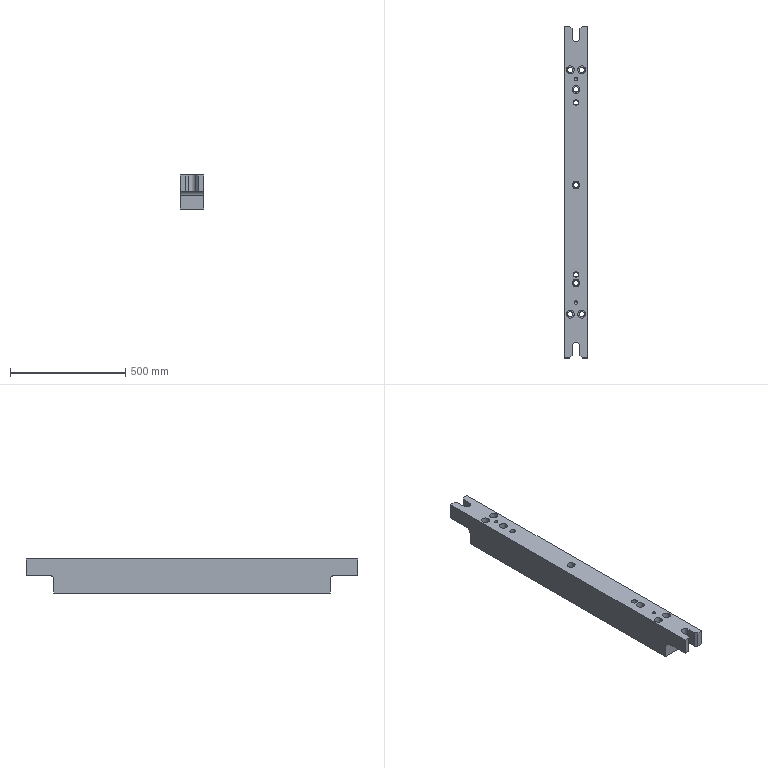Part | STEP file | lll_id2470_x_t | 1 solid | 55 faces | box 100 x 1440 x 147.5 mm | volume 18182535 mm3 | plane 29 | cylinder 24 | cone 2 | commonest cylinder face diameters 23.009 x7 34.008 x7 14.506 x2 20 x2 24 x2 34 x2
STEP:
#1=CARTESIAN_POINT('',(3774.688,-480.,370.));
#2=VERTEX_POINT('',#1);
#3=CARTESIAN_POINT('',(3767.435,-480.,370.));
#4=DIRECTION('',(0.,0.,-1.));
#5=DIRECTION('',(1.,0.,0.));
#6=AXIS2_PLACEMENT_3D('',#3,#4,#5);
#7=CIRCLE('',#6,7.253);
#8=EDGE_CURVE('',#2,#2,#7,.T.);
#9=ORIENTED_EDGE('',*,*,#8,.T.);
#10=EDGE_LOOP('',(#9));
#11=FACE_BOUND('',#10,.T.);
#12=CARTESIAN_POINT('',(3750.431,-395.,370.));
#13=VERTEX_POINT('',#12);
#14=CARTESIAN_POINT('',(3767.435,-395.,370.));
#15=DIRECTION('',(0.,0.,-1.));
#16=DIRECTION('',(-1.,0.,0.));
#17=AXIS2_PLACEMENT_3D('',#14,#15,#16);
#18=CIRCLE('',#17,17.004);
#19=EDGE_CURVE('',#13,#13,#18,.T.);
#20=ORIENTED_EDGE('',*,*,#19,.T.);
#21=EDGE_LOOP('',(#20));
#22=FACE_BOUND('',#21,.T.);
#23=CARTESIAN_POINT('',(3775.431,-530.,370.));
#24=VERTEX_POINT('',#23);
#25=CARTESIAN_POINT('',(3792.435,-530.,370.));
#26=DIRECTION('',(0.,0.,-1.));
#27=DIRECTION('',(-1.,0.,0.));
#28=AXIS2_PLACEMENT_3D('',#25,#26,#27);
#29=CIRCLE('',#28,17.004);
#30=EDGE_CURVE('',#24,#24,#29,.T.);
#31=ORIENTED_EDGE('',*,*,#30,.T.);
#32=EDGE_LOOP('',(#31));
#33=FACE_BOUND('',#32,.T.);
#34=CARTESIAN_POINT('',(3725.431,-530.,370.));
#35=VERTEX_POINT('',#34);
#36=CARTESIAN_POINT('',(3742.435,-530.,370.));
#37=DIRECTION('',(0.,0.,-1.));
#38=DIRECTION('',(-1.,0.,0.));
#39=AXIS2_PLACEMENT_3D('',#36,#37,#38);
#40=CIRCLE('',#39,17.004);
#41=EDGE_CURVE('',#35,#35,#40,.T.);
#42=ORIENTED_EDGE('',*,*,#41,.T.);
#43=EDGE_LOOP('',(#42));
#44=FACE_BOUND('',#43,.T.);
#45=CARTESIAN_POINT('',(3755.435,388.,370.));
#46=VERTEX_POINT('',#45);
#47=CARTESIAN_POINT('',(3767.435,388.,370.));
#48=DIRECTION('',(0.,0.,-1.));
#49=DIRECTION('',(-1.,0.,0.));
#50=AXIS2_PLACEMENT_3D('',#47,#48,#49);
#51=CIRCLE('',#50,12.);
#52=EDGE_CURVE('',#46,#46,#51,.T.);
#53=ORIENTED_EDGE('',*,*,#52,.T.);
#54=EDGE_LOOP('',(#53));
#55=FACE_BOUND('',#54,.T.);
#56=CARTESIAN_POINT('',(3784.439,30.,370.));
#57=VERTEX_POINT('',#56);
#58=CARTESIAN_POINT('',(3767.435,30.,370.));
#59=DIRECTION('',(0.,0.,-1.));
#60=DIRECTION('',(1.,0.,0.));
#61=AXIS2_PLACEMENT_3D('',#58,#59,#60);
#62=CIRCLE('',#61,17.004);
#63=EDGE_CURVE('',#57,#57,#62,.T.);
#64=ORIENTED_EDGE('',*,*,#63,.T.);
#65=EDGE_LOOP('',(#64));
#66=FACE_BOUND('',#65,.T.);
#67=CARTESIAN_POINT('',(3784.439,445.,370.));
#68=VERTEX_POINT('',#67);
#69=CARTESIAN_POINT('',(3767.435,445.,370.));
#70=DIRECTION('',(0.,0.,-1.));
#71=DIRECTION('',(1.,0.,0.));
#72=AXIS2_PLACEMENT_3D('',#69,#70,#71);
#73=CIRCLE('',#72,17.004);
#74=EDGE_CURVE('',#68,#68,#73,.T.);
#75=ORIENTED_EDGE('',*,*,#74,.T.);
#76=EDGE_LOOP('',(#75));
#77=FACE_BOUND('',#76,.T.);
#78=CARTESIAN_POINT('',(3740.435,-720.,370.));
#79=VERTEX_POINT('',#78);
#80=CARTESIAN_POINT('',(3717.435,-720.,370.));
#81=VERTEX_POINT('',#80);
#82=CARTESIAN_POINT('',(1551.12,-720.,370.));
#83=DIRECTION('',(-1.,0.,0.));
#84=VECTOR('',#83,1.);
#85=LINE('',#82,#84);
#86=EDGE_CURVE('',#79,#81,#85,.T.);
#87=ORIENTED_EDGE('',*,*,#86,.F.);
#88=CARTESIAN_POINT('',(3750.435,-710.,370.));
#89=VERTEX_POINT('',#88);
#90=CARTESIAN_POINT('',(3750.435,-710.,370.));
#91=DIRECTION('',(0.7071,0.7071,0.));
#92=VECTOR('',#91,1.);
#93=LINE('',#90,#92);
#94=EDGE_CURVE('',#79,#89,#93,.T.);
#95=ORIENTED_EDGE('',*,*,#94,.T.);
#96=CARTESIAN_POINT('',(3750.435,-670.,370.));
#97=VERTEX_POINT('',#96);
#98=CARTESIAN_POINT('',(3750.435,120.,370.));
#99=DIRECTION('',(0.,-1.,0.));
#100=VECTOR('',#99,1.);
#101=LINE('',#98,#100);
#102=EDGE_CURVE('',#97,#89,#101,.T.);
#103=ORIENTED_EDGE('',*,*,#102,.F.);
#104=CARTESIAN_POINT('',(3784.435,-670.,370.));
#105=VERTEX_POINT('',#104);
#106=CARTESIAN_POINT('',(3767.435,-670.,370.));
#107=DIRECTION('',(0.,0.,1.));
#108=DIRECTION('',(1.,0.,0.));
#109=AXIS2_PLACEMENT_3D('',#106,#107,#108);
#110=CIRCLE('',#109,17.);
#111=EDGE_CURVE('',#105,#97,#110,.T.);
#112=ORIENTED_EDGE('',*,*,#111,.F.);
#113=CARTESIAN_POINT('',(3784.435,-710.,370.));
#114=VERTEX_POINT('',#113);
#115=CARTESIAN_POINT('',(3784.435,120.,370.));
#116=DIRECTION('',(0.,1.,0.));
#117=VECTOR('',#116,1.);
#118=LINE('',#115,#117);
#119=EDGE_CURVE('',#114,#105,#118,.T.);
#120=ORIENTED_EDGE('',*,*,#119,.F.);
#121=CARTESIAN_POINT('',(3794.435,-720.,370.));
#122=VERTEX_POINT('',#121);
#123=CARTESIAN_POINT('',(3784.435,-710.,370.));
#124=DIRECTION('',(0.7071,-0.7071,0.));
#125=VECTOR('',#124,1.);
#126=LINE('',#123,#125);
#127=EDGE_CURVE('',#114,#122,#126,.T.);
#128=ORIENTED_EDGE('',*,*,#127,.T.);
#129=CARTESIAN_POINT('',(3817.435,-720.,370.));
#130=VERTEX_POINT('',#129);
#131=CARTESIAN_POINT('',(1551.12,-720.,370.));
#132=DIRECTION('',(-1.,0.,0.));
#133=VECTOR('',#132,1.);
#134=LINE('',#131,#133);
#135=EDGE_CURVE('',#130,#122,#134,.T.);
#136=ORIENTED_EDGE('',*,*,#135,.F.);
#137=CARTESIAN_POINT('',(3817.435,720.,370.));
#138=VERTEX_POINT('',#137);
#139=CARTESIAN_POINT('',(3817.435,0.,370.));
#140=DIRECTION('',(0.,-1.,0.));
#141=VECTOR('',#140,1.);
#142=LINE('',#139,#141);
#143=EDGE_CURVE('',#138,#130,#142,.T.);
#144=ORIENTED_EDGE('',*,*,#143,.F.);
#145=CARTESIAN_POINT('',(3794.435,720.,370.));
#146=VERTEX_POINT('',#145);
#147=CARTESIAN_POINT('',(1551.12,720.,370.));
#148=DIRECTION('',(1.,0.,0.));
#149=VECTOR('',#148,1.);
#150=LINE('',#147,#149);
#151=EDGE_CURVE('',#146,#138,#150,.T.);
#152=ORIENTED_EDGE('',*,*,#151,.F.);
#153=CARTESIAN_POINT('',(3784.435,710.,370.));
#154=VERTEX_POINT('',#153);
#155=CARTESIAN_POINT('',(3750.935,676.5,370.));
#156=DIRECTION('',(0.7071,0.7071,0.));
#157=VECTOR('',#156,1.);
#158=LINE('',#155,#157);
#159=EDGE_CURVE('',#154,#146,#158,.T.);
#160=ORIENTED_EDGE('',*,*,#159,.F.);
#161=CARTESIAN_POINT('',(3784.435,670.,370.));
#162=VERTEX_POINT('',#161);
#163=CARTESIAN_POINT('',(3784.435,-120.,370.));
#164=DIRECTION('',(0.,-1.,0.));
#165=VECTOR('',#164,1.);
#166=LINE('',#163,#165);
#167=EDGE_CURVE('',#154,#162,#166,.T.);
#168=ORIENTED_EDGE('',*,*,#167,.T.);
#169=CARTESIAN_POINT('',(3750.435,670.,370.));
#170=VERTEX_POINT('',#169);
#171=CARTESIAN_POINT('',(3767.435,670.,370.));
#172=DIRECTION('',(0.,0.,-1.));
#173=DIRECTION('',(1.,0.,0.));
#174=AXIS2_PLACEMENT_3D('',#171,#172,#173);
#175=CIRCLE('',#174,17.);
#176=EDGE_CURVE('',#162,#170,#175,.T.);
#177=ORIENTED_EDGE('',*,*,#176,.T.);
#178=CARTESIAN_POINT('',(3750.435,710.,370.));
#179=VERTEX_POINT('',#178);
#180=CARTESIAN_POINT('',(3750.435,-120.,370.));
#181=DIRECTION('',(0.,1.,0.));
#182=VECTOR('',#181,1.);
#183=LINE('',#180,#182);
#184=EDGE_CURVE('',#170,#179,#183,.T.);
#185=ORIENTED_EDGE('',*,*,#184,.T.);
#186=CARTESIAN_POINT('',(3740.435,720.,370.));
#187=VERTEX_POINT('',#186);
#188=CARTESIAN_POINT('',(4443.935,16.5,370.));
#189=DIRECTION('',(0.7071,-0.7071,0.));
#190=VECTOR('',#189,1.);
#191=LINE('',#188,#190);
#192=EDGE_CURVE('',#187,#179,#191,.T.);
#193=ORIENTED_EDGE('',*,*,#192,.F.);
#194=CARTESIAN_POINT('',(3717.435,720.,370.));
#195=VERTEX_POINT('',#194);
#196=CARTESIAN_POINT('',(1551.12,720.,370.));
#197=DIRECTION('',(1.,0.,0.));
#198=VECTOR('',#197,1.);
#199=LINE('',#196,#198);
#200=EDGE_CURVE('',#195,#187,#199,.T.);
#201=ORIENTED_EDGE('',*,*,#200,.F.);
#202=CARTESIAN_POINT('',(3717.435,-1.,370.));
#203=DIRECTION('',(0.,1.,0.));
#204=VECTOR('',#203,1.);
#205=LINE('',#202,#204);
#206=EDGE_CURVE('',#81,#195,#205,.T.);
#207=ORIENTED_EDGE('',*,*,#206,.F.);
#208=EDGE_LOOP('',(#87,#95,#103,#112,#120,#128,#136,#144,#152,#160,#168,#177,#185,#193,#201,#207));
#209=FACE_BOUND('',#208,.T.);
#210=CARTESIAN_POINT('',(3755.435,-358.,370.));
#211=VERTEX_POINT('',#210);
#212=CARTESIAN_POINT('',(3767.435,-358.,370.));
#213=DIRECTION('',(0.,0.,-1.));
#214=DIRECTION('',(-1.,0.,0.));
#215=AXIS2_PLACEMENT_3D('',#212,#213,#214);
#216=CIRCLE('',#215,12.);
#217=EDGE_CURVE('',#211,#211,#216,.T.);
#218=ORIENTED_EDGE('',*,*,#217,.T.);
#219=EDGE_LOOP('',(#218));
#220=FACE_BOUND('',#219,.T.);
#221=CARTESIAN_POINT('',(3759.439,530.,370.));
#222=VERTEX_POINT('',#221);
#223=CARTESIAN_POINT('',(3742.435,530.,370.));
#224=DIRECTION('',(0.,0.,-1.));
#225=DIRECTION('',(1.,0.,0.));
#226=AXIS2_PLACEMENT_3D('',#223,#224,#225);
#227=CIRCLE('',#226,17.004);
#228=EDGE_CURVE('',#222,#222,#227,.T.);
#229=ORIENTED_EDGE('',*,*,#228,.T.);
#230=EDGE_LOOP('',(#229));
#231=FACE_BOUND('',#230,.T.);
#232=CARTESIAN_POINT('',(3775.431,530.,370.));
#233=VERTEX_POINT('',#232);
#234=CARTESIAN_POINT('',(3792.435,530.,370.));
#235=DIRECTION('',(0.,0.,1.));
#236=DIRECTION('',(-1.,0.,0.));
#237=AXIS2_PLACEMENT_3D('',#234,#235,#236);
#238=CIRCLE('',#237,17.004);
#239=EDGE_CURVE('',#233,#233,#238,.T.);
#240=ORIENTED_EDGE('',*,*,#239,.F.);
#241=EDGE_LOOP('',(#240));
#242=FACE_BOUND('',#241,.T.);
#243=CARTESIAN_POINT('',(3774.688,490.,370.));
#244=VERTEX_POINT('',#243);
#245=CARTESIAN_POINT('',(3767.435,490.,370.));
#246=DIRECTION('',(0.,0.,-1.));
#247=DIRECTION('',(1.,0.,0.));
#248=AXIS2_PLACEMENT_3D('',#245,#246,#247);
#249=CIRCLE('',#248,7.253);
#250=EDGE_CURVE('',#244,#244,#249,.T.);
#251=ORIENTED_EDGE('',*,*,#250,.T.);
#252=EDGE_LOOP('',(#251));
#253=FACE_BOUND('',#252,.T.);
#254=CARTESIAN_POINT('',(1551.12,-1.,370.));
#255=DIRECTION('',(0.,0.,-1.));
#256=DIRECTION('',(1.,0.,0.));
#257=AXIS2_PLACEMENT_3D('',#254,#255,#256);
#258=PLANE('',#257);
#259=ADVANCED_FACE('',(#11,#22,#33,#44,#55,#66,#77,#209,#220,#231,#242,#253),#258,.F.);
#260=CARTESIAN_POINT('',(3817.435,600.,280.));
#261=VERTEX_POINT('',#260);
#262=CARTESIAN_POINT('',(3817.435,620.,300.));
#263=VERTEX_POINT('',#262);
#264=CARTESIAN_POINT('',(3817.435,620.,280.));
#265=DIRECTION('',(-1.,0.,0.));
#266=DIRECTION('',(0.,0.,-1.));
#267=AXIS2_PLACEMENT_3D('',#264,#265,#266);
#268=CIRCLE('',#267,20.);
#269=EDGE_CURVE('',#261,#263,#268,.T.);
#270=ORIENTED_EDGE('',*,*,#269,.F.);
#271=CARTESIAN_POINT('',(3717.435,600.,280.));
#272=VERTEX_POINT('',#271);
#273=CARTESIAN_POINT('',(3807.435,600.,280.));
#274=DIRECTION('',(1.,0.,0.));
#275=VECTOR('',#274,1.);
#276=LINE('',#273,#275);
#277=EDGE_CURVE('',#272,#261,#276,.T.);
#278=ORIENTED_EDGE('',*,*,#277,.F.);
#279=CARTESIAN_POINT('',(3717.435,620.,300.));
#280=VERTEX_POINT('',#279);
#281=CARTESIAN_POINT('',(3717.435,620.,280.));
#282=DIRECTION('',(1.,0.,0.));
#283=DIRECTION('',(0.,0.,-1.));
#284=AXIS2_PLACEMENT_3D('',#281,#282,#283);
#285=CIRCLE('',#284,20.);
#286=EDGE_CURVE('',#280,#272,#285,.T.);
#287=ORIENTED_EDGE('',*,*,#286,.F.);
#288=CARTESIAN_POINT('',(3727.435,620.,300.));
#289=DIRECTION('',(-1.,0.,0.));
#290=VECTOR('',#289,1.);
#291=LINE('',#288,#290);
#292=EDGE_CURVE('',#263,#280,#291,.T.);
#293=ORIENTED_EDGE('',*,*,#292,.F.);
#294=EDGE_LOOP('',(#270,#278,#287,#293));
#295=FACE_OUTER_BOUND('',#294,.T.);
#296=CARTESIAN_POINT('',(3767.435,620.,280.));
#297=DIRECTION('',(1.,0.,0.));
#298=DIRECTION('',(0.,0.,1.));
#299=AXIS2_PLACEMENT_3D('',#296,#297,#298);
#300=CYLINDRICAL_SURFACE('',#299,20.);
#301=ADVANCED_FACE('',(#295),#300,.F.);
#302=CARTESIAN_POINT('',(3817.435,720.,300.));
#303=VERTEX_POINT('',#302);
#304=CARTESIAN_POINT('',(3817.435,-641.5,300.));
#305=DIRECTION('',(0.,1.,0.));
#306=VECTOR('',#305,1.);
#307=LINE('',#304,#306);
#308=EDGE_CURVE('',#263,#303,#307,.T.);
#309=ORIENTED_EDGE('',*,*,#308,.F.);
#310=ORIENTED_EDGE('',*,*,#292,.T.);
#311=CARTESIAN_POINT('',(3717.435,720.,300.));
#312=VERTEX_POINT('',#311);
#313=CARTESIAN_POINT('',(3717.435,-641.5,300.));
#314=DIRECTION('',(0.,1.,0.));
#315=VECTOR('',#314,1.);
#316=LINE('',#313,#315);
#317=EDGE_CURVE('',#280,#312,#316,.T.);
#318=ORIENTED_EDGE('',*,*,#317,.T.);
#319=CARTESIAN_POINT('',(3740.435,720.,300.));
#320=VERTEX_POINT('',#319);
#321=CARTESIAN_POINT('',(3767.435,720.,300.));
#322=DIRECTION('',(1.,0.,0.));
#323=VECTOR('',#322,1.);
#324=LINE('',#321,#323);
#325=EDGE_CURVE('',#312,#320,#324,.T.);
#326=ORIENTED_EDGE('',*,*,#325,.T.);
#327=CARTESIAN_POINT('',(3750.435,710.,300.));
#328=VERTEX_POINT('',#327);
#329=CARTESIAN_POINT('',(3740.435,720.,300.));
#330=DIRECTION('',(0.7071,-0.7071,0.));
#331=VECTOR('',#330,1.);
#332=LINE('',#329,#331);
#333=EDGE_CURVE('',#320,#328,#332,.T.);
#334=ORIENTED_EDGE('',*,*,#333,.T.);
#335=CARTESIAN_POINT('',(3750.435,670.,300.));
#336=VERTEX_POINT('',#335);
#337=CARTESIAN_POINT('',(3750.435,-641.5,300.));
#338=DIRECTION('',(0.,-1.,0.));
#339=VECTOR('',#338,1.);
#340=LINE('',#337,#339);
#341=EDGE_CURVE('',#328,#336,#340,.T.);
#342=ORIENTED_EDGE('',*,*,#341,.T.);
#343=CARTESIAN_POINT('',(3784.435,670.,300.));
#344=VERTEX_POINT('',#343);
#345=CARTESIAN_POINT('',(3767.435,670.,300.));
#346=DIRECTION('',(0.,0.,-1.));
#347=DIRECTION('',(-1.,0.,0.));
#348=AXIS2_PLACEMENT_3D('',#345,#346,#347);
#349=CIRCLE('',#348,17.);
#350=EDGE_CURVE('',#344,#336,#349,.T.);
#351=ORIENTED_EDGE('',*,*,#350,.F.);
#352=CARTESIAN_POINT('',(3784.435,710.,300.));
#353=VERTEX_POINT('',#352);
#354=CARTESIAN_POINT('',(3784.435,-641.5,300.));
#355=DIRECTION('',(0.,1.,0.));
#356=VECTOR('',#355,1.);
#357=LINE('',#354,#356);
#358=EDGE_CURVE('',#344,#353,#357,.T.);
#359=ORIENTED_EDGE('',*,*,#358,.T.);
#360=CARTESIAN_POINT('',(3794.435,720.,300.));
#361=VERTEX_POINT('',#360);
#362=CARTESIAN_POINT('',(3794.435,720.,300.));
#363=DIRECTION('',(0.7071,0.7071,0.));
#364=VECTOR('',#363,1.);
#365=LINE('',#362,#364);
#366=EDGE_CURVE('',#353,#361,#365,.T.);
#367=ORIENTED_EDGE('',*,*,#366,.T.);
#368=CARTESIAN_POINT('',(3767.435,720.,300.));
#369=DIRECTION('',(1.,0.,0.));
#370=VECTOR('',#369,1.);
#371=LINE('',#368,#370);
#372=EDGE_CURVE('',#361,#303,#371,.T.);
#373=ORIENTED_EDGE('',*,*,#372,.T.);
#374=EDGE_LOOP('',(#309,#310,#318,#326,#334,#342,#351,#359,#367,#373));
#375=FACE_OUTER_BOUND('',#374,.T.);
#376=CARTESIAN_POINT('',(3767.435,-641.5,300.));
#377=DIRECTION('',(0.,0.,-1.));
#378=DIRECTION('',(1.,0.,0.));
#379=AXIS2_PLACEMENT_3D('',#376,#377,#378);
#380=PLANE('',#379);
#381=ADVANCED_FACE('',(#375),#380,.T.);
#382=CARTESIAN_POINT('',(3750.435,-710.,300.));
#383=VERTEX_POINT('',#382);
#384=CARTESIAN_POINT('',(3750.435,-670.,300.));
#385=VERTEX_POINT('',#384);
#386=CARTESIAN_POINT('',(3750.435,-661.5,300.));
#387=DIRECTION('',(0.,1.,0.));
#388=VECTOR('',#387,1.);
#389=LINE('',#386,#388);
#390=EDGE_CURVE('',#383,#385,#389,.T.);
#391=ORIENTED_EDGE('',*,*,#390,.F.);
#392=CARTESIAN_POINT('',(3740.435,-720.,300.));
#393=VERTEX_POINT('',#392);
#394=CARTESIAN_POINT('',(3773.185,-687.25,300.));
#395=DIRECTION('',(-0.7071,-0.7071,0.));
#396=VECTOR('',#395,1.);
#397=LINE('',#394,#396);
#398=EDGE_CURVE('',#383,#393,#397,.T.);
#399=ORIENTED_EDGE('',*,*,#398,.T.);
#400=CARTESIAN_POINT('',(3717.435,-720.,300.));
#401=VERTEX_POINT('',#400);
#402=CARTESIAN_POINT('',(3767.435,-720.,300.));
#403=DIRECTION('',(-1.,0.,0.));
#404=VECTOR('',#403,1.);
#405=LINE('',#402,#404);
#406=EDGE_CURVE('',#393,#401,#405,.T.);
#407=ORIENTED_EDGE('',*,*,#406,.T.);
#408=CARTESIAN_POINT('',(3717.435,-620.,300.));
#409=VERTEX_POINT('',#408);
#410=CARTESIAN_POINT('',(3717.435,-681.5,300.));
#411=DIRECTION('',(0.,1.,0.));
#412=VECTOR('',#411,1.);
#413=LINE('',#410,#412);
#414=EDGE_CURVE('',#401,#409,#413,.T.);
#415=ORIENTED_EDGE('',*,*,#414,.T.);
#416=CARTESIAN_POINT('',(3817.435,-620.,300.));
#417=VERTEX_POINT('',#416);
#418=CARTESIAN_POINT('',(3807.435,-620.,300.));
#419=DIRECTION('',(1.,0.,0.));
#420=VECTOR('',#419,1.);
#421=LINE('',#418,#420);
#422=EDGE_CURVE('',#409,#417,#421,.T.);
#423=ORIENTED_EDGE('',*,*,#422,.T.);
#424=CARTESIAN_POINT('',(3817.435,-720.,300.));
#425=VERTEX_POINT('',#424);
#426=CARTESIAN_POINT('',(3817.435,-681.5,300.));
#427=DIRECTION('',(0.,1.,0.));
#428=VECTOR('',#427,1.);
#429=LINE('',#426,#428);
#430=EDGE_CURVE('',#425,#417,#429,.T.);
#431=ORIENTED_EDGE('',*,*,#430,.F.);
#432=CARTESIAN_POINT('',(3794.435,-720.,300.));
#433=VERTEX_POINT('',#432);
#434=CARTESIAN_POINT('',(3767.435,-720.,300.));
#435=DIRECTION('',(-1.,0.,0.));
#436=VECTOR('',#435,1.);
#437=LINE('',#434,#436);
#438=EDGE_CURVE('',#425,#433,#437,.T.);
#439=ORIENTED_EDGE('',*,*,#438,.T.);
#440=CARTESIAN_POINT('',(3784.435,-710.,300.));
#441=VERTEX_POINT('',#440);
#442=CARTESIAN_POINT('',(3761.685,-687.25,300.));
#443=DIRECTION('',(-0.7071,0.7071,0.));
#444=VECTOR('',#443,1.);
#445=LINE('',#442,#444);
#446=EDGE_CURVE('',#433,#441,#445,.T.);
#447=ORIENTED_EDGE('',*,*,#446,.T.);
#448=CARTESIAN_POINT('',(3784.435,-670.,300.));
#449=VERTEX_POINT('',#448);
#450=CARTESIAN_POINT('',(3784.435,-661.5,300.));
#451=DIRECTION('',(0.,-1.,0.));
#452=VECTOR('',#451,1.);
#453=LINE('',#450,#452);
#454=EDGE_CURVE('',#449,#441,#453,.T.);
#455=ORIENTED_EDGE('',*,*,#454,.F.);
#456=CARTESIAN_POINT('',(3767.435,-670.,300.));
#457=DIRECTION('',(0.,0.,1.));
#458=DIRECTION('',(1.,0.,0.));
#459=AXIS2_PLACEMENT_3D('',#456,#457,#458);
#460=CIRCLE('',#459,17.);
#461=EDGE_CURVE('',#449,#385,#460,.T.);
#462=ORIENTED_EDGE('',*,*,#461,.T.);
#463=EDGE_LOOP('',(#391,#399,#407,#415,#423,#431,#439,#447,#455,#462));
#464=FACE_OUTER_BOUND('',#463,.T.);
#465=CARTESIAN_POINT('',(3767.435,-681.5,300.));
#466=DIRECTION('',(0.,0.,-1.));
#467=DIRECTION('',(1.,0.,0.));
#468=AXIS2_PLACEMENT_3D('',#465,#466,#467);
#469=PLANE('',#468);
#470=ADVANCED_FACE('',(#464),#469,.T.);
#471=CARTESIAN_POINT('',(3717.435,-600.,280.));
#472=VERTEX_POINT('',#471);
#473=CARTESIAN_POINT('',(3717.435,-620.,280.));
#474=DIRECTION('',(1.,0.,0.));
#475=DIRECTION('',(0.,0.,-1.));
#476=AXIS2_PLACEMENT_3D('',#473,#474,#475);
#477=CIRCLE('',#476,20.);
#478=EDGE_CURVE('',#472,#409,#477,.T.);
#479=ORIENTED_EDGE('',*,*,#478,.F.);
#480=CARTESIAN_POINT('',(3817.435,-600.,280.));
#481=VERTEX_POINT('',#480);
#482=CARTESIAN_POINT('',(3727.435,-600.,280.));
#483=DIRECTION('',(-1.,0.,0.));
#484=VECTOR('',#483,1.);
#485=LINE('',#482,#484);
#486=EDGE_CURVE('',#481,#472,#485,.T.);
#487=ORIENTED_EDGE('',*,*,#486,.F.);
#488=CARTESIAN_POINT('',(3817.435,-620.,280.));
#489=DIRECTION('',(-1.,0.,0.));
#490=DIRECTION('',(0.,0.,-1.));
#491=AXIS2_PLACEMENT_3D('',#488,#489,#490);
#492=CIRCLE('',#491,20.);
#493=EDGE_CURVE('',#417,#481,#492,.T.);
#494=ORIENTED_EDGE('',*,*,#493,.F.);
#495=ORIENTED_EDGE('',*,*,#422,.F.);
#496=EDGE_LOOP('',(#479,#487,#494,#495));
#497=FACE_OUTER_BOUND('',#496,.T.);
#498=CARTESIAN_POINT('',(3767.435,-620.,280.));
#499=DIRECTION('',(-1.,0.,0.));
#500=DIRECTION('',(0.,0.,-1.));
#501=AXIS2_PLACEMENT_3D('',#498,#499,#500);
#502=CYLINDRICAL_SURFACE('',#501,20.);
#503=ADVANCED_FACE('',(#497),#502,.F.);
#504=CARTESIAN_POINT('',(3755.435,-358.,270.));
#505=VERTEX_POINT('',#504);
#506=CARTESIAN_POINT('',(3767.435,-358.,270.));
#507=DIRECTION('',(0.,0.,-1.));
#508=DIRECTION('',(-1.,0.,0.));
#509=AXIS2_PLACEMENT_3D('',#506,#507,#508);
#510=CIRCLE('',#509,12.);
#511=EDGE_CURVE('',#505,#505,#510,.T.);
#512=ORIENTED_EDGE('',*,*,#511,.F.);
#513=EDGE_LOOP('',(#512));
#514=FACE_BOUND('',#513,.T.);
#515=CARTESIAN_POINT('',(3777.435,-358.,270.));
#516=VERTEX_POINT('',#515);
#517=CARTESIAN_POINT('',(3767.435,-358.,270.));
#518=DIRECTION('',(0.,0.,1.));
#519=DIRECTION('',(1.,0.,0.));
#520=AXIS2_PLACEMENT_3D('',#517,#518,#519);
#521=CIRCLE('',#520,10.);
#522=EDGE_CURVE('',#516,#516,#521,.T.);
#523=ORIENTED_EDGE('',*,*,#522,.F.);
#524=EDGE_LOOP('',(#523));
#525=FACE_BOUND('',#524,.T.);
#526=CARTESIAN_POINT('',(3767.435,-358.,270.));
#527=DIRECTION('',(0.,0.,-1.));
#528=DIRECTION('',(1.,0.,0.));
#529=AXIS2_PLACEMENT_3D('',#526,#527,#528);
#530=PLANE('',#529);
#531=ADVANCED_FACE('',(#514,#525),#530,.F.);
#532=CARTESIAN_POINT('',(3730.931,530.,272.5));
#533=VERTEX_POINT('',#532);
#534=CARTESIAN_POINT('',(3742.435,530.,272.5));
#535=DIRECTION('',(0.,0.,-1.));
#536=DIRECTION('',(-1.,0.,0.));
#537=AXIS2_PLACEMENT_3D('',#534,#535,#536);
#538=CIRCLE('',#537,11.505);
#539=EDGE_CURVE('',#533,#533,#538,.T.);
#540=ORIENTED_EDGE('',*,*,#539,.T.);
#541=EDGE_LOOP('',(#540));
#542=FACE_BOUND('',#541,.T.);
#543=CARTESIAN_POINT('',(3759.439,530.,272.5));
#544=VERTEX_POINT('',#543);
#545=CARTESIAN_POINT('',(3742.435,530.,272.5));
#546=DIRECTION('',(0.,0.,-1.));
#547=DIRECTION('',(1.,0.,0.));
#548=AXIS2_PLACEMENT_3D('',#545,#546,#547);
#549=CIRCLE('',#548,17.004);
#550=EDGE_CURVE('',#544,#544,#549,.T.);
#551=ORIENTED_EDGE('',*,*,#550,.F.);
#552=EDGE_LOOP('',(#551));
#553=FACE_BOUND('',#552,.T.);
#554=CARTESIAN_POINT('',(3742.435,530.,272.5));
#555=DIRECTION('',(0.,0.,-1.));
#556=DIRECTION('',(-1.,0.,0.));
#557=AXIS2_PLACEMENT_3D('',#554,#555,#556);
#558=PLANE('',#557);
#559=ADVANCED_FACE('',(#542,#553),#558,.F.);
#560=CARTESIAN_POINT('',(3803.94,530.,272.5));
#561=VERTEX_POINT('',#560);
#562=CARTESIAN_POINT('',(3792.435,530.,272.5));
#563=DIRECTION('',(0.,0.,1.));
#564=DIRECTION('',(1.,0.,0.));
#565=AXIS2_PLACEMENT_3D('',#562,#563,#564);
#566=CIRCLE('',#565,11.505);
#567=EDGE_CURVE('',#561,#561,#566,.T.);
#568=ORIENTED_EDGE('',*,*,#567,.F.);
#569=EDGE_LOOP('',(#568));
#570=FACE_BOUND('',#569,.T.);
#571=CARTESIAN_POINT('',(3775.431,530.,272.5));
#572=VERTEX_POINT('',#571);
#573=CARTESIAN_POINT('',(3792.435,530.,272.5));
#574=DIRECTION('',(0.,0.,1.));
#575=DIRECTION('',(-1.,0.,0.));
#576=AXIS2_PLACEMENT_3D('',#573,#574,#575);
#577=CIRCLE('',#576,17.004);
#578=EDGE_CURVE('',#572,#572,#577,.T.);
#579=ORIENTED_EDGE('',*,*,#578,.T.);
#580=EDGE_LOOP('',(#579));
#581=FACE_BOUND('',#580,.T.);
#582=CARTESIAN_POINT('',(3792.435,530.,272.5));
#583=DIRECTION('',(0.,0.,-1.));
#584=DIRECTION('',(1.,0.,0.));
#585=AXIS2_PLACEMENT_3D('',#582,#583,#584);
#586=PLANE('',#585);
#587=ADVANCED_FACE('',(#570,#581),#586,.F.);
#588=CARTESIAN_POINT('',(3755.931,445.,272.5));
#589=VERTEX_POINT('',#588);
#590=CARTESIAN_POINT('',(3767.435,445.,272.5));
#591=DIRECTION('',(0.,0.,-1.));
#592=DIRECTION('',(-1.,0.,0.));
#593=AXIS2_PLACEMENT_3D('',#590,#591,#592);
#594=CIRCLE('',#593,11.505);
#595=EDGE_CURVE('',#589,#589,#594,.T.);
#596=ORIENTED_EDGE('',*,*,#595,.T.);
#597=EDGE_LOOP('',(#596));
#598=FACE_BOUND('',#597,.T.);
#599=CARTESIAN_POINT('',(3784.439,445.,272.5));
#600=VERTEX_POINT('',#599);
#601=CARTESIAN_POINT('',(3767.435,445.,272.5));
#602=DIRECTION('',(0.,0.,-1.));
#603=DIRECTION('',(1.,0.,0.));
#604=AXIS2_PLACEMENT_3D('',#601,#602,#603);
#605=CIRCLE('',#604,17.004);
#606=EDGE_CURVE('',#600,#600,#605,.T.);
#607=ORIENTED_EDGE('',*,*,#606,.F.);
#608=EDGE_LOOP('',(#607));
#609=FACE_BOUND('',#608,.T.);
#610=CARTESIAN_POINT('',(3767.435,445.,272.5));
#611=DIRECTION('',(0.,0.,-1.));
#612=DIRECTION('',(-1.,0.,0.));
#613=AXIS2_PLACEMENT_3D('',#610,#611,#612);
#614=PLANE('',#613);
#615=ADVANCED_FACE('',(#598,#609),#614,.F.);
#616=CARTESIAN_POINT('',(3755.931,30.,272.5));
#617=VERTEX_POINT('',#616);
#618=CARTESIAN_POINT('',(3767.435,30.,272.5));
#619=DIRECTION('',(0.,0.,-1.));
#620=DIRECTION('',(-1.,0.,0.));
#621=AXIS2_PLACEMENT_3D('',#618,#619,#620);
#622=CIRCLE('',#621,11.505);
#623=EDGE_CURVE('',#617,#617,#622,.T.);
#624=ORIENTED_EDGE('',*,*,#623,.T.);
#625=EDGE_LOOP('',(#624));
#626=FACE_BOUND('',#625,.T.);
#627=CARTESIAN_POINT('',(3784.439,30.,272.5));
#628=VERTEX_POINT('',#627);
#629=CARTESIAN_POINT('',(3767.435,30.,272.5));
#630=DIRECTION('',(0.,0.,-1.));
#631=DIRECTION('',(1.,0.,0.));
#632=AXIS2_PLACEMENT_3D('',#629,#630,#631);
#633=CIRCLE('',#632,17.004);
#634=EDGE_CURVE('',#628,#628,#633,.T.);
#635=ORIENTED_EDGE('',*,*,#634,.F.);
#636=EDGE_LOOP('',(#635));
#637=FACE_BOUND('',#636,.T.);
#638=CARTESIAN_POINT('',(3767.435,0.,272.5));
#639=DIRECTION('',(0.,0.,-1.));
#640=DIRECTION('',(-1.,0.,0.));
#641=AXIS2_PLACEMENT_3D('',#638,#639,#640);
#642=PLANE('',#641);
#643=ADVANCED_FACE('',(#626,#637),#642,.F.);
#644=CARTESIAN_POINT('',(3755.435,388.,270.));
#645=VERTEX_POINT('',#644);
#646=CARTESIAN_POINT('',(3767.435,388.,270.));
#647=DIRECTION('',(0.,0.,1.));
#648=DIRECTION('',(-1.,0.,0.));
#649=AXIS2_PLACEMENT_3D('',#646,#647,#648);
#650=CIRCLE('',#649,12.);
#651=EDGE_CURVE('',#645,#645,#650,.T.);
#652=ORIENTED_EDGE('',*,*,#651,.T.);
#653=EDGE_LOOP('',(#652));
#654=FACE_BOUND('',#653,.T.);
#655=CARTESIAN_POINT('',(3777.435,388.,270.));
#656=VERTEX_POINT('',#655);
#657=CARTESIAN_POINT('',(3767.435,388.,270.));
#658=DIRECTION('',(0.,0.,-1.));
#659=DIRECTION('',(1.,0.,0.));
#660=AXIS2_PLACEMENT_3D('',#657,#658,#659);
#661=CIRCLE('',#660,10.);
#662=EDGE_CURVE('',#656,#656,#661,.T.);
#663=ORIENTED_EDGE('',*,*,#662,.T.);
#664=EDGE_LOOP('',(#663));
#665=FACE_BOUND('',#664,.T.);
#666=CARTESIAN_POINT('',(3767.435,388.,270.));
#667=DIRECTION('',(0.,0.,-1.));
#668=DIRECTION('',(1.,0.,0.));
#669=AXIS2_PLACEMENT_3D('',#666,#667,#668);
#670=PLANE('',#669);
#671=ADVANCED_FACE('',(#654,#665),#670,.F.);
#672=ORIENTED_EDGE('',*,*,#578,.F.);
#673=EDGE_LOOP('',(#672));
#674=FACE_BOUND('',#673,.T.);
#675=ORIENTED_EDGE('',*,*,#239,.T.);
#676=EDGE_LOOP('',(#675));
#677=FACE_BOUND('',#676,.T.);
#678=CARTESIAN_POINT('',(3792.435,530.,370.));
#679=DIRECTION('',(0.,0.,-1.));
#680=DIRECTION('',(-1.,0.,0.));
#681=AXIS2_PLACEMENT_3D('',#678,#679,#680);
#682=CYLINDRICAL_SURFACE('',#681,17.004);
#683=ADVANCED_FACE('',(#674,#677),#682,.F.);
#684=ORIENTED_EDGE('',*,*,#550,.T.);
#685=EDGE_LOOP('',(#684));
#686=FACE_BOUND('',#685,.T.);
#687=ORIENTED_EDGE('',*,*,#228,.F.);
#688=EDGE_LOOP('',(#687));
#689=FACE_BOUND('',#688,.T.);
#690=CARTESIAN_POINT('',(3742.435,530.,370.));
#691=DIRECTION('',(0.,0.,-1.));
#692=DIRECTION('',(1.,0.,0.));
#693=AXIS2_PLACEMENT_3D('',#690,#691,#692);
#694=CYLINDRICAL_SURFACE('',#693,17.004);
#695=ADVANCED_FACE('',(#686,#689),#694,.F.);
#696=ORIENTED_EDGE('',*,*,#511,.T.);
#697=EDGE_LOOP('',(#696));
#698=FACE_BOUND('',#697,.T.);
#699=ORIENTED_EDGE('',*,*,#217,.F.);
#700=EDGE_LOOP('',(#699));
#701=FACE_BOUND('',#700,.T.);
#702=CARTESIAN_POINT('',(3767.435,-358.,370.));
#703=DIRECTION('',(0.,0.,-1.));
#704=DIRECTION('',(-1.,0.,0.));
#705=AXIS2_PLACEMENT_3D('',#702,#703,#704);
#706=CYLINDRICAL_SURFACE('',#705,12.);
#707=ADVANCED_FACE('',(#698,#701),#706,.F.);
#708=ORIENTED_EDGE('',*,*,#184,.F.);
#709=CARTESIAN_POINT('',(3750.435,670.,370.));
#710=DIRECTION('',(0.,0.,-1.));
#711=VECTOR('',#710,1.);
#712=LINE('',#709,#711);
#713=EDGE_CURVE('',#170,#336,#712,.T.);
#714=ORIENTED_EDGE('',*,*,#713,.T.);
#715=ORIENTED_EDGE('',*,*,#341,.F.);
#716=CARTESIAN_POINT('',(3750.435,710.,385.));
#717=DIRECTION('',(0.,0.,-1.));
#718=VECTOR('',#717,1.);
#719=LINE('',#716,#718);
#720=EDGE_CURVE('',#179,#328,#719,.T.);
#721=ORIENTED_EDGE('',*,*,#720,.F.);
#722=EDGE_LOOP('',(#708,#714,#715,#721));
#723=FACE_OUTER_BOUND('',#722,.T.);
#724=CARTESIAN_POINT('',(3750.435,-720.,385.));
#725=DIRECTION('',(1.,0.,0.));
#726=DIRECTION('',(0.,0.,-1.));
#727=AXIS2_PLACEMENT_3D('',#724,#725,#726);
#728=PLANE('',#727);
#729=ADVANCED_FACE('',(#723),#728,.T.);
#730=ORIENTED_EDGE('',*,*,#713,.F.);
#731=ORIENTED_EDGE('',*,*,#176,.F.);
#732=CARTESIAN_POINT('',(3784.435,670.,370.));
#733=DIRECTION('',(0.,0.,1.));
#734=VECTOR('',#733,1.);
#735=LINE('',#732,#734);
#736=EDGE_CURVE('',#344,#162,#735,.T.);
#737=ORIENTED_EDGE('',*,*,#736,.F.);
#738=ORIENTED_EDGE('',*,*,#350,.T.);
#739=EDGE_LOOP('',(#730,#731,#737,#738));
#740=FACE_OUTER_BOUND('',#739,.T.);
#741=CARTESIAN_POINT('',(3767.435,670.,345.));
#742=DIRECTION('',(0.,0.,-1.));
#743=DIRECTION('',(-1.,0.,0.));
#744=AXIS2_PLACEMENT_3D('',#741,#742,#743);
#745=CYLINDRICAL_SURFACE('',#744,17.);
#746=ADVANCED_FACE('',(#740),#745,.F.);
#747=ORIENTED_EDGE('',*,*,#358,.F.);
#748=ORIENTED_EDGE('',*,*,#736,.T.);
#749=ORIENTED_EDGE('',*,*,#167,.F.);
#750=CARTESIAN_POINT('',(3784.435,710.,385.));
#751=DIRECTION('',(0.,0.,1.));
#752=VECTOR('',#751,1.);
#753=LINE('',#750,#752);
#754=EDGE_CURVE('',#353,#154,#753,.T.);
#755=ORIENTED_EDGE('',*,*,#754,.F.);
#756=EDGE_LOOP('',(#747,#748,#749,#755));
#757=FACE_OUTER_BOUND('',#756,.T.);
#758=CARTESIAN_POINT('',(3784.435,-720.,385.));
#759=DIRECTION('',(-1.,0.,0.));
#760=DIRECTION('',(0.,0.,1.));
#761=AXIS2_PLACEMENT_3D('',#758,#759,#760);
#762=PLANE('',#761);
#763=ADVANCED_FACE('',(#757),#762,.T.);
#764=ORIENTED_EDGE('',*,*,#159,.T.);
#765=CARTESIAN_POINT('',(3794.435,720.,-450.));
#766=DIRECTION('',(0.,0.,-1.));
#767=VECTOR('',#766,1.);
#768=LINE('',#765,#767);
#769=EDGE_CURVE('',#146,#361,#768,.T.);
#770=ORIENTED_EDGE('',*,*,#769,.T.);
#771=ORIENTED_EDGE('',*,*,#366,.F.);
#772=ORIENTED_EDGE('',*,*,#754,.T.);
#773=EDGE_LOOP('',(#764,#770,#771,#772));
#774=FACE_OUTER_BOUND('',#773,.T.);
#775=CARTESIAN_POINT('',(3794.435,720.,-450.));
#776=DIRECTION('',(0.7071,-0.7071,0.));
#777=DIRECTION('',(0.,0.,-1.));
#778=AXIS2_PLACEMENT_3D('',#775,#776,#777);
#779=PLANE('',#778);
#780=ADVANCED_FACE('',(#774),#779,.F.);
#781=ORIENTED_EDGE('',*,*,#769,.F.);
#782=ORIENTED_EDGE('',*,*,#151,.T.);
#783=CARTESIAN_POINT('',(3817.435,720.,241.25));
#784=DIRECTION('',(0.,0.,-1.));
#785=VECTOR('',#784,1.);
#786=LINE('',#783,#785);
#787=EDGE_CURVE('',#138,#303,#786,.T.);
#788=ORIENTED_EDGE('',*,*,#787,.T.);
#789=ORIENTED_EDGE('',*,*,#372,.F.);
#790=EDGE_LOOP('',(#781,#782,#788,#789));
#791=FACE_OUTER_BOUND('',#790,.T.);
#792=CARTESIAN_POINT('',(3737.435,720.,310.));
#793=DIRECTION('',(0.,1.,0.));
#794=DIRECTION('',(0.,0.,-1.));
#795=AXIS2_PLACEMENT_3D('',#792,#793,#794);
#796=PLANE('',#795);
#797=ADVANCED_FACE('',(#791),#796,.T.);
#798=ORIENTED_EDGE('',*,*,#135,.T.);
#799=CARTESIAN_POINT('',(3794.435,-720.,310.));
#800=DIRECTION('',(0.,0.,-1.));
#801=VECTOR('',#800,1.);
#802=LINE('',#799,#801);
#803=EDGE_CURVE('',#122,#433,#802,.T.);
#804=ORIENTED_EDGE('',*,*,#803,.T.);
#805=ORIENTED_EDGE('',*,*,#438,.F.);
#806=CARTESIAN_POINT('',(3817.435,-720.,241.25));
#807=DIRECTION('',(0.,0.,1.));
#808=VECTOR('',#807,1.);
#809=LINE('',#806,#808);
#810=EDGE_CURVE('',#425,#130,#809,.T.);
#811=ORIENTED_EDGE('',*,*,#810,.T.);
#812=EDGE_LOOP('',(#798,#804,#805,#811));
#813=FACE_OUTER_BOUND('',#812,.T.);
#814=CARTESIAN_POINT('',(7707.435,-720.,310.));
#815=DIRECTION('',(0.,-1.,0.));
#816=DIRECTION('',(0.,0.,1.));
#817=AXIS2_PLACEMENT_3D('',#814,#815,#816);
#818=PLANE('',#817);
#819=ADVANCED_FACE('',(#813),#818,.T.);
#820=ORIENTED_EDGE('',*,*,#454,.T.);
#821=CARTESIAN_POINT('',(3784.435,-710.,385.));
#822=DIRECTION('',(0.,0.,1.));
#823=VECTOR('',#822,1.);
#824=LINE('',#821,#823);
#825=EDGE_CURVE('',#441,#114,#824,.T.);
#826=ORIENTED_EDGE('',*,*,#825,.T.);
#827=ORIENTED_EDGE('',*,*,#119,.T.);
#828=CARTESIAN_POINT('',(3784.435,-670.,370.));
#829=DIRECTION('',(0.,0.,1.));
#830=VECTOR('',#829,1.);
#831=LINE('',#828,#830);
#832=EDGE_CURVE('',#449,#105,#831,.T.);
#833=ORIENTED_EDGE('',*,*,#832,.F.);
#834=EDGE_LOOP('',(#820,#826,#827,#833));
#835=FACE_OUTER_BOUND('',#834,.T.);
#836=CARTESIAN_POINT('',(3784.435,720.,385.));
#837=DIRECTION('',(-1.,0.,0.));
#838=DIRECTION('',(0.,0.,1.));
#839=AXIS2_PLACEMENT_3D('',#836,#837,#838);
#840=PLANE('',#839);
#841=ADVANCED_FACE('',(#835),#840,.T.);
#842=CARTESIAN_POINT('',(3750.435,-670.,370.));
#843=DIRECTION('',(0.,0.,-1.));
#844=VECTOR('',#843,1.);
#845=LINE('',#842,#844);
#846=EDGE_CURVE('',#97,#385,#845,.T.);
#847=ORIENTED_EDGE('',*,*,#846,.T.);
#848=ORIENTED_EDGE('',*,*,#461,.F.);
#849=ORIENTED_EDGE('',*,*,#832,.T.);
#850=ORIENTED_EDGE('',*,*,#111,.T.);
#851=EDGE_LOOP('',(#847,#848,#849,#850));
#852=FACE_OUTER_BOUND('',#851,.T.);
#853=CARTESIAN_POINT('',(3767.435,-670.,345.));
#854=DIRECTION('',(0.,0.,-1.));
#855=DIRECTION('',(-1.,0.,0.));
#856=AXIS2_PLACEMENT_3D('',#853,#854,#855);
#857=CYLINDRICAL_SURFACE('',#856,17.);
#858=ADVANCED_FACE('',(#852),#857,.F.);
#859=ORIENTED_EDGE('',*,*,#102,.T.);
#860=CARTESIAN_POINT('',(3750.435,-710.,385.));
#861=DIRECTION('',(0.,0.,-1.));
#862=VECTOR('',#861,1.);
#863=LINE('',#860,#862);
#864=EDGE_CURVE('',#89,#383,#863,.T.);
#865=ORIENTED_EDGE('',*,*,#864,.T.);
#866=ORIENTED_EDGE('',*,*,#390,.T.);
#867=ORIENTED_EDGE('',*,*,#846,.F.);
#868=EDGE_LOOP('',(#859,#865,#866,#867));
#869=FACE_OUTER_BOUND('',#868,.T.);
#870=CARTESIAN_POINT('',(3750.435,720.,385.));
#871=DIRECTION('',(1.,0.,0.));
#872=DIRECTION('',(0.,0.,-1.));
#873=AXIS2_PLACEMENT_3D('',#870,#871,#872);
#874=PLANE('',#873);
#875=ADVANCED_FACE('',(#869),#874,.T.);
#876=ORIENTED_EDGE('',*,*,#406,.F.);
#877=CARTESIAN_POINT('',(3740.435,-720.,310.));
#878=DIRECTION('',(0.,0.,1.));
#879=VECTOR('',#878,1.);
#880=LINE('',#877,#879);
#881=EDGE_CURVE('',#393,#79,#880,.T.);
#882=ORIENTED_EDGE('',*,*,#881,.T.);
#883=ORIENTED_EDGE('',*,*,#86,.T.);
#884=CARTESIAN_POINT('',(3717.435,-720.,310.));
#885=DIRECTION('',(0.,0.,-1.));
#886=VECTOR('',#885,1.);
#887=LINE('',#884,#886);
#888=EDGE_CURVE('',#81,#401,#887,.T.);
#889=ORIENTED_EDGE('',*,*,#888,.T.);
#890=EDGE_LOOP('',(#876,#882,#883,#889));
#891=FACE_OUTER_BOUND('',#890,.T.);
#892=CARTESIAN_POINT('',(7707.435,-720.,310.));
#893=DIRECTION('',(0.,-1.,0.));
#894=DIRECTION('',(0.,0.,1.));
#895=AXIS2_PLACEMENT_3D('',#892,#893,#894);
#896=PLANE('',#895);
#897=ADVANCED_FACE('',(#891),#896,.T.);
#898=CARTESIAN_POINT('',(3817.435,-600.,222.5));
#899=VERTEX_POINT('',#898);
#900=CARTESIAN_POINT('',(3817.435,-600.,271.25));
#901=DIRECTION('',(0.,0.,-1.));
#902=VECTOR('',#901,1.);
#903=LINE('',#900,#902);
#904=EDGE_CURVE('',#481,#899,#903,.T.);
#905=ORIENTED_EDGE('',*,*,#904,.F.);
#906=ORIENTED_EDGE('',*,*,#486,.T.);
#907=CARTESIAN_POINT('',(3717.435,-600.,222.5));
#908=VERTEX_POINT('',#907);
#909=CARTESIAN_POINT('',(3717.435,-600.,271.25));
#910=DIRECTION('',(0.,0.,-1.));
#911=VECTOR('',#910,1.);
#912=LINE('',#909,#911);
#913=EDGE_CURVE('',#472,#908,#912,.T.);
#914=ORIENTED_EDGE('',*,*,#913,.T.);
#915=CARTESIAN_POINT('',(1551.12,-600.,222.5));
#916=DIRECTION('',(-1.,0.,0.));
#917=VECTOR('',#916,1.);
#918=LINE('',#915,#917);
#919=EDGE_CURVE('',#899,#908,#918,.T.);
#920=ORIENTED_EDGE('',*,*,#919,.F.);
#921=EDGE_LOOP('',(#905,#906,#914,#920));
#922=FACE_OUTER_BOUND('',#921,.T.);
#923=CARTESIAN_POINT('',(3767.435,-600.,271.25));
#924=DIRECTION('',(0.,-1.,0.));
#925=DIRECTION('',(0.,0.,1.));
#926=AXIS2_PLACEMENT_3D('',#923,#924,#925);
#927=PLANE('',#926);
#928=ADVANCED_FACE('',(#922),#927,.T.);
#929=CARTESIAN_POINT('',(3817.435,600.,222.5));
#930=VERTEX_POINT('',#929);
#931=CARTESIAN_POINT('',(3817.435,600.,241.25));
#932=DIRECTION('',(0.,0.,-1.));
#933=VECTOR('',#932,1.);
#934=LINE('',#931,#933);
#935=EDGE_CURVE('',#261,#930,#934,.T.);
#936=ORIENTED_EDGE('',*,*,#935,.F.);
#937=ORIENTED_EDGE('',*,*,#269,.T.);
#938=ORIENTED_EDGE('',*,*,#308,.T.);
#939=ORIENTED_EDGE('',*,*,#787,.F.);
#940=ORIENTED_EDGE('',*,*,#143,.T.);
#941=ORIENTED_EDGE('',*,*,#810,.F.);
#942=ORIENTED_EDGE('',*,*,#430,.T.);
#943=ORIENTED_EDGE('',*,*,#493,.T.);
#944=ORIENTED_EDGE('',*,*,#904,.T.);
#945=CARTESIAN_POINT('',(3817.435,-1.,222.5));
#946=DIRECTION('',(0.,1.,0.));
#947=VECTOR('',#946,1.);
#948=LINE('',#945,#947);
#949=EDGE_CURVE('',#899,#930,#948,.T.);
#950=ORIENTED_EDGE('',*,*,#949,.T.);
#951=EDGE_LOOP('',(#936,#937,#938,#939,#940,#941,#942,#943,#944,#950));
#952=FACE_OUTER_BOUND('',#951,.T.);
#953=CARTESIAN_POINT('',(3817.435,0.,241.25));
#954=DIRECTION('',(-1.,0.,0.));
#955=DIRECTION('',(0.,0.,-1.));
#956=AXIS2_PLACEMENT_3D('',#953,#954,#955);
#957=PLANE('',#956);
#958=ADVANCED_FACE('',(#952),#957,.F.);
#959=CARTESIAN_POINT('',(3717.435,600.,222.5));
#960=VERTEX_POINT('',#959);
#961=CARTESIAN_POINT('',(3717.435,600.,271.25));
#962=DIRECTION('',(0.,0.,1.));
#963=VECTOR('',#962,1.);
#964=LINE('',#961,#963);
#965=EDGE_CURVE('',#960,#272,#964,.T.);
#966=ORIENTED_EDGE('',*,*,#965,.T.);
#967=ORIENTED_EDGE('',*,*,#277,.T.);
#968=ORIENTED_EDGE('',*,*,#935,.T.);
#969=CARTESIAN_POINT('',(1551.12,600.,222.5));
#970=DIRECTION('',(1.,0.,0.));
#971=VECTOR('',#970,1.);
#972=LINE('',#969,#971);
#973=EDGE_CURVE('',#960,#930,#972,.T.);
#974=ORIENTED_EDGE('',*,*,#973,.F.);
#975=EDGE_LOOP('',(#966,#967,#968,#974));
#976=FACE_OUTER_BOUND('',#975,.T.);
#977=CARTESIAN_POINT('',(3767.435,600.,271.25));
#978=DIRECTION('',(0.,1.,0.));
#979=DIRECTION('',(0.,0.,-1.));
#980=AXIS2_PLACEMENT_3D('',#977,#978,#979);
#981=PLANE('',#980);
#982=ADVANCED_FACE('',(#976),#981,.T.);
#983=ORIENTED_EDGE('',*,*,#965,.F.);
#984=CARTESIAN_POINT('',(3717.435,-1.,222.5));
#985=DIRECTION('',(0.,1.,0.));
#986=VECTOR('',#985,1.);
#987=LINE('',#984,#986);
#988=EDGE_CURVE('',#908,#960,#987,.T.);
#989=ORIENTED_EDGE('',*,*,#988,.F.);
#990=ORIENTED_EDGE('',*,*,#913,.F.);
#991=ORIENTED_EDGE('',*,*,#478,.T.);
#992=ORIENTED_EDGE('',*,*,#414,.F.);
#993=ORIENTED_EDGE('',*,*,#888,.F.);
#994=ORIENTED_EDGE('',*,*,#206,.T.);
#995=CARTESIAN_POINT('',(3717.435,720.,310.));
#996=DIRECTION('',(0.,0.,-1.));
#997=VECTOR('',#996,1.);
#998=LINE('',#995,#997);
#999=EDGE_CURVE('',#195,#312,#998,.T.);
#1000=ORIENTED_EDGE('',*,*,#999,.T.);
#1001=ORIENTED_EDGE('',*,*,#317,.F.);
#1002=ORIENTED_EDGE('',*,*,#286,.T.);
#1003=EDGE_LOOP('',(#983,#989,#990,#991,#992,#993,#994,#1000,#1001,#1002));
#1004=FACE_OUTER_BOUND('',#1003,.T.);
#1005=CARTESIAN_POINT('',(3717.435,-600.,310.));
#1006=DIRECTION('',(-1.,0.,0.));
#1007=DIRECTION('',(0.,0.,-1.));
#1008=AXIS2_PLACEMENT_3D('',#1005,#1006,#1007);
#1009=PLANE('',#1008);
#1010=ADVANCED_FACE('',(#1004),#1009,.T.);
#1011=ORIENTED_EDGE('',*,*,#522,.T.);
#1012=EDGE_LOOP('',(#1011));
#1013=FACE_BOUND('',#1012,.T.);
#1014=CARTESIAN_POINT('',(3777.435,-358.,222.5));
#1015=VERTEX_POINT('',#1014);
#1016=CARTESIAN_POINT('',(3767.435,-358.,222.5));
#1017=DIRECTION('',(0.,0.,-1.));
#1018=DIRECTION('',(1.,0.,0.));
#1019=AXIS2_PLACEMENT_3D('',#1016,#1017,#1018);
#1020=CIRCLE('',#1019,10.);
#1021=EDGE_CURVE('',#1015,#1015,#1020,.T.);
#1022=ORIENTED_EDGE('',*,*,#1021,.T.);
#1023=EDGE_LOOP('',(#1022));
#1024=FACE_BOUND('',#1023,.T.);
#1025=CARTESIAN_POINT('',(3767.435,-358.,420.));
#1026=DIRECTION('',(0.,0.,-1.));
#1027=DIRECTION('',(-1.,0.,0.));
#1028=AXIS2_PLACEMENT_3D('',#1025,#1026,#1027);
#1029=CYLINDRICAL_SURFACE('',#1028,10.);
#1030=ADVANCED_FACE('',(#1013,#1024),#1029,.F.);
#1031=CARTESIAN_POINT('',(3753.94,530.,222.5));
#1032=VERTEX_POINT('',#1031);
#1033=CARTESIAN_POINT('',(3742.435,530.,222.5));
#1034=DIRECTION('',(0.,0.,-1.));
#1035=DIRECTION('',(1.,0.,0.));
#1036=AXIS2_PLACEMENT_3D('',#1033,#1034,#1035);
#1037=CIRCLE('',#1036,11.505);
#1038=EDGE_CURVE('',#1032,#1032,#1037,.T.);
#1039=ORIENTED_EDGE('',*,*,#1038,.T.);
#1040=EDGE_LOOP('',(#1039));
#1041=FACE_BOUND('',#1040,.T.);
#1042=ORIENTED_EDGE('',*,*,#539,.F.);
#1043=EDGE_LOOP('',(#1042));
#1044=FACE_BOUND('',#1043,.T.);
#1045=CARTESIAN_POINT('',(3742.435,530.,422.));
#1046=DIRECTION('',(0.,0.,-1.));
#1047=DIRECTION('',(1.,0.,0.));
#1048=AXIS2_PLACEMENT_3D('',#1045,#1046,#1047);
#1049=CYLINDRICAL_SURFACE('',#1048,11.505);
#1050=ADVANCED_FACE('',(#1041,#1044),#1049,.F.);
#1051=CARTESIAN_POINT('',(3803.94,530.,222.5));
#1052=VERTEX_POINT('',#1051);
#1053=CARTESIAN_POINT('',(3792.435,530.,222.5));
#1054=DIRECTION('',(0.,0.,-1.));
#1055=DIRECTION('',(1.,0.,0.));
#1056=AXIS2_PLACEMENT_3D('',#1053,#1054,#1055);
#1057=CIRCLE('',#1056,11.505);
#1058=EDGE_CURVE('',#1052,#1052,#1057,.T.);
#1059=ORIENTED_EDGE('',*,*,#1058,.T.);
#1060=EDGE_LOOP('',(#1059));
#1061=FACE_BOUND('',#1060,.T.);
#1062=ORIENTED_EDGE('',*,*,#567,.T.);
#1063=EDGE_LOOP('',(#1062));
#1064=FACE_BOUND('',#1063,.T.);
#1065=CARTESIAN_POINT('',(3792.435,530.,422.));
#1066=DIRECTION('',(0.,0.,-1.));
#1067=DIRECTION('',(-1.,0.,0.));
#1068=AXIS2_PLACEMENT_3D('',#1065,#1066,#1067);
#1069=CYLINDRICAL_SURFACE('',#1068,11.505);
#1070=ADVANCED_FACE('',(#1061,#1064),#1069,.F.);
#1071=CARTESIAN_POINT('',(3778.94,445.,222.5));
#1072=VERTEX_POINT('',#1071);
#1073=CARTESIAN_POINT('',(3767.435,445.,222.5));
#1074=DIRECTION('',(0.,0.,-1.));
#1075=DIRECTION('',(1.,0.,0.));
#1076=AXIS2_PLACEMENT_3D('',#1073,#1074,#1075);
#1077=CIRCLE('',#1076,11.505);
#1078=EDGE_CURVE('',#1072,#1072,#1077,.T.);
#1079=ORIENTED_EDGE('',*,*,#1078,.T.);
#1080=EDGE_LOOP('',(#1079));
#1081=FACE_BOUND('',#1080,.T.);
#1082=ORIENTED_EDGE('',*,*,#595,.F.);
#1083=EDGE_LOOP('',(#1082));
#1084=FACE_BOUND('',#1083,.T.);
#1085=CARTESIAN_POINT('',(3767.435,445.,422.));
#1086=DIRECTION('',(0.,0.,-1.));
#1087=DIRECTION('',(1.,0.,0.));
#1088=AXIS2_PLACEMENT_3D('',#1085,#1086,#1087);
#1089=CYLINDRICAL_SURFACE('',#1088,11.505);
#1090=ADVANCED_FACE('',(#1081,#1084),#1089,.F.);
#1091=CARTESIAN_POINT('',(3778.94,30.,222.5));
#1092=VERTEX_POINT('',#1091);
#1093=CARTESIAN_POINT('',(3767.435,30.,222.5));
#1094=DIRECTION('',(0.,0.,-1.));
#1095=DIRECTION('',(1.,0.,0.));
#1096=AXIS2_PLACEMENT_3D('',#1093,#1094,#1095);
#1097=CIRCLE('',#1096,11.505);
#1098=EDGE_CURVE('',#1092,#1092,#1097,.T.);
#1099=ORIENTED_EDGE('',*,*,#1098,.T.);
#1100=EDGE_LOOP('',(#1099));
#1101=FACE_BOUND('',#1100,.T.);
#1102=ORIENTED_EDGE('',*,*,#623,.F.);
#1103=EDGE_LOOP('',(#1102));
#1104=FACE_BOUND('',#1103,.T.);
#1105=CARTESIAN_POINT('',(3767.435,30.,422.));
#1106=DIRECTION('',(0.,0.,-1.));
#1107=DIRECTION('',(1.,0.,0.));
#1108=AXIS2_PLACEMENT_3D('',#1105,#1106,#1107);
#1109=CYLINDRICAL_SURFACE('',#1108,11.505);
#1110=ADVANCED_FACE('',(#1101,#1104),#1109,.F.);
#1111=ORIENTED_EDGE('',*,*,#662,.F.);
#1112=EDGE_LOOP('',(#1111));
#1113=FACE_BOUND('',#1112,.T.);
#1114=CARTESIAN_POINT('',(3777.435,388.,222.5));
#1115=VERTEX_POINT('',#1114);
#1116=CARTESIAN_POINT('',(3767.435,388.,222.5));
#1117=DIRECTION('',(0.,0.,1.));
#1118=DIRECTION('',(1.,0.,0.));
#1119=AXIS2_PLACEMENT_3D('',#1116,#1117,#1118);
#1120=CIRCLE('',#1119,10.);
#1121=EDGE_CURVE('',#1115,#1115,#1120,.T.);
#1122=ORIENTED_EDGE('',*,*,#1121,.F.);
#1123=EDGE_LOOP('',(#1122));
#1124=FACE_BOUND('',#1123,.T.);
#1125=CARTESIAN_POINT('',(3767.435,388.,420.));
#1126=DIRECTION('',(0.,0.,-1.));
#1127=DIRECTION('',(-1.,0.,0.));
#1128=AXIS2_PLACEMENT_3D('',#1125,#1126,#1127);
#1129=CYLINDRICAL_SURFACE('',#1128,10.);
#1130=ADVANCED_FACE('',(#1113,#1124),#1129,.F.);
#1131=CARTESIAN_POINT('',(3755.931,-395.,222.5));
#1132=VERTEX_POINT('',#1131);
#1133=CARTESIAN_POINT('',(3767.435,-395.,222.5));
#1134=DIRECTION('',(0.,0.,-1.));
#1135=DIRECTION('',(-1.,0.,0.));
#1136=AXIS2_PLACEMENT_3D('',#1133,#1134,#1135);
#1137=CIRCLE('',#1136,11.505);
#1138=EDGE_CURVE('',#1132,#1132,#1137,.T.);
#1139=ORIENTED_EDGE('',*,*,#1138,.F.);
#1140=EDGE_LOOP('',(#1139));
#1141=FACE_BOUND('',#1140,.T.);
#1142=CARTESIAN_POINT('',(3780.931,-530.,222.5));
#1143=VERTEX_POINT('',#1142);
#1144=CARTESIAN_POINT('',(3792.435,-530.,222.5));
#1145=DIRECTION('',(0.,0.,-1.));
#1146=DIRECTION('',(-1.,0.,0.));
#1147=AXIS2_PLACEMENT_3D('',#1144,#1145,#1146);
#1148=CIRCLE('',#1147,11.505);
#1149=EDGE_CURVE('',#1143,#1143,#1148,.T.);
#1150=ORIENTED_EDGE('',*,*,#1149,.F.);
#1151=EDGE_LOOP('',(#1150));
#1152=FACE_BOUND('',#1151,.T.);
#1153=CARTESIAN_POINT('',(3730.931,-530.,222.5));
#1154=VERTEX_POINT('',#1153);
#1155=CARTESIAN_POINT('',(3742.435,-530.,222.5));
#1156=DIRECTION('',(0.,0.,-1.));
#1157=DIRECTION('',(-1.,0.,0.));
#1158=AXIS2_PLACEMENT_3D('',#1155,#1156,#1157);
#1159=CIRCLE('',#1158,11.505);
#1160=EDGE_CURVE('',#1154,#1154,#1159,.T.);
#1161=ORIENTED_EDGE('',*,*,#1160,.F.);
#1162=EDGE_LOOP('',(#1161));
#1163=FACE_BOUND('',#1162,.T.);
#1164=ORIENTED_EDGE('',*,*,#1121,.T.);
#1165=EDGE_LOOP('',(#1164));
#1166=FACE_BOUND('',#1165,.T.);
#1167=ORIENTED_EDGE('',*,*,#1098,.F.);
#1168=EDGE_LOOP('',(#1167));
#1169=FACE_BOUND('',#1168,.T.);
#1170=ORIENTED_EDGE('',*,*,#1078,.F.);
#1171=EDGE_LOOP('',(#1170));
#1172=FACE_BOUND('',#1171,.T.);
#1173=ORIENTED_EDGE('',*,*,#1058,.F.);
#1174=EDGE_LOOP('',(#1173));
#1175=FACE_BOUND('',#1174,.T.);
#1176=ORIENTED_EDGE('',*,*,#1038,.F.);
#1177=EDGE_LOOP('',(#1176));
#1178=FACE_BOUND('',#1177,.T.);
#1179=ORIENTED_EDGE('',*,*,#1021,.F.);
#1180=EDGE_LOOP('',(#1179));
#1181=FACE_BOUND('',#1180,.T.);
#1182=ORIENTED_EDGE('',*,*,#988,.T.);
#1183=ORIENTED_EDGE('',*,*,#973,.T.);
#1184=ORIENTED_EDGE('',*,*,#949,.F.);
#1185=ORIENTED_EDGE('',*,*,#919,.T.);
#1186=EDGE_LOOP('',(#1182,#1183,#1184,#1185));
#1187=FACE_BOUND('',#1186,.T.);
#1188=CARTESIAN_POINT('',(1551.12,-1.,222.5));
#1189=DIRECTION('',(0.,0.,-1.));
#1190=DIRECTION('',(1.,0.,0.));
#1191=AXIS2_PLACEMENT_3D('',#1188,#1189,#1190);
#1192=PLANE('',#1191);
#1193=ADVANCED_FACE('',(#1141,#1152,#1163,#1166,#1169,#1172,#1175,#1178,#1181,#1187),#1192,.T.);
#1194=CARTESIAN_POINT('',(3740.435,720.,-450.));
#1195=DIRECTION('',(0.,0.,1.));
#1196=VECTOR('',#1195,1.);
#1197=LINE('',#1194,#1196);
#1198=EDGE_CURVE('',#320,#187,#1197,.T.);
#1199=ORIENTED_EDGE('',*,*,#1198,.F.);
#1200=ORIENTED_EDGE('',*,*,#325,.F.);
#1201=ORIENTED_EDGE('',*,*,#999,.F.);
#1202=ORIENTED_EDGE('',*,*,#200,.T.);
#1203=EDGE_LOOP('',(#1199,#1200,#1201,#1202));
#1204=FACE_OUTER_BOUND('',#1203,.T.);
#1205=CARTESIAN_POINT('',(3737.435,720.,310.));
#1206=DIRECTION('',(0.,1.,0.));
#1207=DIRECTION('',(0.,0.,-1.));
#1208=AXIS2_PLACEMENT_3D('',#1205,#1206,#1207);
#1209=PLANE('',#1208);
#1210=ADVANCED_FACE('',(#1204),#1209,.T.);
#1211=ORIENTED_EDGE('',*,*,#333,.F.);
#1212=ORIENTED_EDGE('',*,*,#1198,.T.);
#1213=ORIENTED_EDGE('',*,*,#192,.T.);
#1214=ORIENTED_EDGE('',*,*,#720,.T.);
#1215=EDGE_LOOP('',(#1211,#1212,#1213,#1214));
#1216=FACE_OUTER_BOUND('',#1215,.T.);
#1217=CARTESIAN_POINT('',(3740.435,720.,-450.));
#1218=DIRECTION('',(-0.7071,-0.7071,0.));
#1219=DIRECTION('',(0.,0.,1.));
#1220=AXIS2_PLACEMENT_3D('',#1217,#1218,#1219);
#1221=PLANE('',#1220);
#1222=ADVANCED_FACE('',(#1216),#1221,.F.);
#1223=ORIENTED_EDGE('',*,*,#606,.T.);
#1224=EDGE_LOOP('',(#1223));
#1225=FACE_BOUND('',#1224,.T.);
#1226=ORIENTED_EDGE('',*,*,#74,.F.);
#1227=EDGE_LOOP('',(#1226));
#1228=FACE_BOUND('',#1227,.T.);
#1229=CARTESIAN_POINT('',(3767.435,445.,370.));
#1230=DIRECTION('',(0.,0.,-1.));
#1231=DIRECTION('',(1.,0.,0.));
#1232=AXIS2_PLACEMENT_3D('',#1229,#1230,#1231);
#1233=CYLINDRICAL_SURFACE('',#1232,17.004);
#1234=ADVANCED_FACE('',(#1225,#1228),#1233,.F.);
#1235=ORIENTED_EDGE('',*,*,#634,.T.);
#1236=EDGE_LOOP('',(#1235));
#1237=FACE_BOUND('',#1236,.T.);
#1238=ORIENTED_EDGE('',*,*,#63,.F.);
#1239=EDGE_LOOP('',(#1238));
#1240=FACE_BOUND('',#1239,.T.);
#1241=CARTESIAN_POINT('',(3767.435,30.,370.));
#1242=DIRECTION('',(0.,0.,-1.));
#1243=DIRECTION('',(1.,0.,0.));
#1244=AXIS2_PLACEMENT_3D('',#1241,#1242,#1243);
#1245=CYLINDRICAL_SURFACE('',#1244,17.004);
#1246=ADVANCED_FACE('',(#1237,#1240),#1245,.F.);
#1247=ORIENTED_EDGE('',*,*,#651,.F.);
#1248=EDGE_LOOP('',(#1247));
#1249=FACE_BOUND('',#1248,.T.);
#1250=ORIENTED_EDGE('',*,*,#52,.F.);
#1251=EDGE_LOOP('',(#1250));
#1252=FACE_BOUND('',#1251,.T.);
#1253=CARTESIAN_POINT('',(3767.435,388.,370.));
#1254=DIRECTION('',(0.,0.,-1.));
#1255=DIRECTION('',(-1.,0.,0.));
#1256=AXIS2_PLACEMENT_3D('',#1253,#1254,#1255);
#1257=CYLINDRICAL_SURFACE('',#1256,12.);
#1258=ADVANCED_FACE('',(#1249,#1252),#1257,.F.);
#1259=CARTESIAN_POINT('',(3730.931,-530.,272.5));
#1260=VERTEX_POINT('',#1259);
#1261=CARTESIAN_POINT('',(3742.435,-530.,272.5));
#1262=DIRECTION('',(0.,0.,-1.));
#1263=DIRECTION('',(-1.,0.,0.));
#1264=AXIS2_PLACEMENT_3D('',#1261,#1262,#1263);
#1265=CIRCLE('',#1264,11.505);
#1266=EDGE_CURVE('',#1260,#1260,#1265,.T.);
#1267=ORIENTED_EDGE('',*,*,#1266,.T.);
#1268=EDGE_LOOP('',(#1267));
#1269=FACE_BOUND('',#1268,.T.);
#1270=CARTESIAN_POINT('',(3759.439,-530.,272.5));
#1271=VERTEX_POINT('',#1270);
#1272=CARTESIAN_POINT('',(3742.435,-530.,272.5));
#1273=DIRECTION('',(0.,0.,-1.));
#1274=DIRECTION('',(1.,0.,0.));
#1275=AXIS2_PLACEMENT_3D('',#1272,#1273,#1274);
#1276=CIRCLE('',#1275,17.004);
#1277=EDGE_CURVE('',#1271,#1271,#1276,.T.);
#1278=ORIENTED_EDGE('',*,*,#1277,.F.);
#1279=EDGE_LOOP('',(#1278));
#1280=FACE_BOUND('',#1279,.T.);
#1281=CARTESIAN_POINT('',(3742.435,-530.,272.5));
#1282=DIRECTION('',(0.,0.,-1.));
#1283=DIRECTION('',(-1.,0.,0.));
#1284=AXIS2_PLACEMENT_3D('',#1281,#1282,#1283);
#1285=PLANE('',#1284);
#1286=ADVANCED_FACE('',(#1269,#1280),#1285,.F.);
#1287=ORIENTED_EDGE('',*,*,#1160,.T.);
#1288=EDGE_LOOP('',(#1287));
#1289=FACE_BOUND('',#1288,.T.);
#1290=ORIENTED_EDGE('',*,*,#1266,.F.);
#1291=EDGE_LOOP('',(#1290));
#1292=FACE_BOUND('',#1291,.T.);
#1293=CARTESIAN_POINT('',(3742.435,-530.,422.));
#1294=DIRECTION('',(0.,0.,-1.));
#1295=DIRECTION('',(1.,0.,0.));
#1296=AXIS2_PLACEMENT_3D('',#1293,#1294,#1295);
#1297=CYLINDRICAL_SURFACE('',#1296,11.505);
#1298=ADVANCED_FACE('',(#1289,#1292),#1297,.F.);
#1299=ORIENTED_EDGE('',*,*,#1277,.T.);
#1300=EDGE_LOOP('',(#1299));
#1301=FACE_BOUND('',#1300,.T.);
#1302=ORIENTED_EDGE('',*,*,#41,.F.);
#1303=EDGE_LOOP('',(#1302));
#1304=FACE_BOUND('',#1303,.T.);
#1305=CARTESIAN_POINT('',(3742.435,-530.,370.));
#1306=DIRECTION('',(0.,0.,-1.));
#1307=DIRECTION('',(1.,0.,0.));
#1308=AXIS2_PLACEMENT_3D('',#1305,#1306,#1307);
#1309=CYLINDRICAL_SURFACE('',#1308,17.004);
#1310=ADVANCED_FACE('',(#1301,#1304),#1309,.F.);
#1311=CARTESIAN_POINT('',(3803.94,-530.,272.5));
#1312=VERTEX_POINT('',#1311);
#1313=CARTESIAN_POINT('',(3792.435,-530.,272.5));
#1314=DIRECTION('',(0.,0.,1.));
#1315=DIRECTION('',(1.,0.,0.));
#1316=AXIS2_PLACEMENT_3D('',#1313,#1314,#1315);
#1317=CIRCLE('',#1316,11.505);
#1318=EDGE_CURVE('',#1312,#1312,#1317,.T.);
#1319=ORIENTED_EDGE('',*,*,#1318,.F.);
#1320=EDGE_LOOP('',(#1319));
#1321=FACE_BOUND('',#1320,.T.);
#1322=CARTESIAN_POINT('',(3775.431,-530.,272.5));
#1323=VERTEX_POINT('',#1322);
#1324=CARTESIAN_POINT('',(3792.435,-530.,272.5));
#1325=DIRECTION('',(0.,0.,1.));
#1326=DIRECTION('',(-1.,0.,0.));
#1327=AXIS2_PLACEMENT_3D('',#1324,#1325,#1326);
#1328=CIRCLE('',#1327,17.004);
#1329=EDGE_CURVE('',#1323,#1323,#1328,.T.);
#1330=ORIENTED_EDGE('',*,*,#1329,.T.);
#1331=EDGE_LOOP('',(#1330));
#1332=FACE_BOUND('',#1331,.T.);
#1333=CARTESIAN_POINT('',(3792.435,-530.,272.5));
#1334=DIRECTION('',(0.,0.,-1.));
#1335=DIRECTION('',(1.,0.,0.));
#1336=AXIS2_PLACEMENT_3D('',#1333,#1334,#1335);
#1337=PLANE('',#1336);
#1338=ADVANCED_FACE('',(#1321,#1332),#1337,.F.);
#1339=ORIENTED_EDGE('',*,*,#1149,.T.);
#1340=EDGE_LOOP('',(#1339));
#1341=FACE_BOUND('',#1340,.T.);
#1342=ORIENTED_EDGE('',*,*,#1318,.T.);
#1343=EDGE_LOOP('',(#1342));
#1344=FACE_BOUND('',#1343,.T.);
#1345=CARTESIAN_POINT('',(3792.435,-530.,422.));
#1346=DIRECTION('',(0.,0.,-1.));
#1347=DIRECTION('',(-1.,0.,0.));
#1348=AXIS2_PLACEMENT_3D('',#1345,#1346,#1347);
#1349=CYLINDRICAL_SURFACE('',#1348,11.505);
#1350=ADVANCED_FACE('',(#1341,#1344),#1349,.F.);
#1351=ORIENTED_EDGE('',*,*,#1329,.F.);
#1352=EDGE_LOOP('',(#1351));
#1353=FACE_BOUND('',#1352,.T.);
#1354=ORIENTED_EDGE('',*,*,#30,.F.);
#1355=EDGE_LOOP('',(#1354));
#1356=FACE_BOUND('',#1355,.T.);
#1357=CARTESIAN_POINT('',(3792.435,-530.,370.));
#1358=DIRECTION('',(0.,0.,-1.));
#1359=DIRECTION('',(-1.,0.,0.));
#1360=AXIS2_PLACEMENT_3D('',#1357,#1358,#1359);
#1361=CYLINDRICAL_SURFACE('',#1360,17.004);
#1362=ADVANCED_FACE('',(#1353,#1356),#1361,.F.);
#1363=CARTESIAN_POINT('',(3755.931,-395.,272.5));
#1364=VERTEX_POINT('',#1363);
#1365=CARTESIAN_POINT('',(3767.435,-395.,272.5));
#1366=DIRECTION('',(0.,0.,-1.));
#1367=DIRECTION('',(-1.,0.,0.));
#1368=AXIS2_PLACEMENT_3D('',#1365,#1366,#1367);
#1369=CIRCLE('',#1368,11.505);
#1370=EDGE_CURVE('',#1364,#1364,#1369,.T.);
#1371=ORIENTED_EDGE('',*,*,#1370,.T.);
#1372=EDGE_LOOP('',(#1371));
#1373=FACE_BOUND('',#1372,.T.);
#1374=CARTESIAN_POINT('',(3784.439,-395.,272.5));
#1375=VERTEX_POINT('',#1374);
#1376=CARTESIAN_POINT('',(3767.435,-395.,272.5));
#1377=DIRECTION('',(0.,0.,-1.));
#1378=DIRECTION('',(1.,0.,0.));
#1379=AXIS2_PLACEMENT_3D('',#1376,#1377,#1378);
#1380=CIRCLE('',#1379,17.004);
#1381=EDGE_CURVE('',#1375,#1375,#1380,.T.);
#1382=ORIENTED_EDGE('',*,*,#1381,.F.);
#1383=EDGE_LOOP('',(#1382));
#1384=FACE_BOUND('',#1383,.T.);
#1385=CARTESIAN_POINT('',(3767.435,-395.,272.5));
#1386=DIRECTION('',(0.,0.,-1.));
#1387=DIRECTION('',(-1.,0.,0.));
#1388=AXIS2_PLACEMENT_3D('',#1385,#1386,#1387);
#1389=PLANE('',#1388);
#1390=ADVANCED_FACE('',(#1373,#1384),#1389,.F.);
#1391=ORIENTED_EDGE('',*,*,#1138,.T.);
#1392=EDGE_LOOP('',(#1391));
#1393=FACE_BOUND('',#1392,.T.);
#1394=ORIENTED_EDGE('',*,*,#1370,.F.);
#1395=EDGE_LOOP('',(#1394));
#1396=FACE_BOUND('',#1395,.T.);
#1397=CARTESIAN_POINT('',(3767.435,-395.,422.));
#1398=DIRECTION('',(0.,0.,-1.));
#1399=DIRECTION('',(1.,0.,0.));
#1400=AXIS2_PLACEMENT_3D('',#1397,#1398,#1399);
#1401=CYLINDRICAL_SURFACE('',#1400,11.505);
#1402=ADVANCED_FACE('',(#1393,#1396),#1401,.F.);
#1403=ORIENTED_EDGE('',*,*,#1381,.T.);
#1404=EDGE_LOOP('',(#1403));
#1405=FACE_BOUND('',#1404,.T.);
#1406=ORIENTED_EDGE('',*,*,#19,.F.);
#1407=EDGE_LOOP('',(#1406));
#1408=FACE_BOUND('',#1407,.T.);
#1409=CARTESIAN_POINT('',(3767.435,-395.,370.));
#1410=DIRECTION('',(0.,0.,-1.));
#1411=DIRECTION('',(1.,0.,0.));
#1412=AXIS2_PLACEMENT_3D('',#1409,#1410,#1411);
#1413=CYLINDRICAL_SURFACE('',#1412,17.004);
#1414=ADVANCED_FACE('',(#1405,#1408),#1413,.F.);
#1415=CARTESIAN_POINT('',(3760.182,490.,332.247));
#1416=VERTEX_POINT('',#1415);
#1417=CARTESIAN_POINT('',(3767.435,490.,332.247));
#1418=DIRECTION('',(0.,0.,-1.));
#1419=DIRECTION('',(-1.,0.,0.));
#1420=AXIS2_PLACEMENT_3D('',#1417,#1418,#1419);
#1421=CIRCLE('',#1420,7.253);
#1422=EDGE_CURVE('',#1416,#1416,#1421,.T.);
#1423=ORIENTED_EDGE('',*,*,#1422,.T.);
#1424=EDGE_LOOP('',(#1423));
#1425=FACE_BOUND('',#1424,.T.);
#1426=ORIENTED_EDGE('',*,*,#250,.F.);
#1427=EDGE_LOOP('',(#1426));
#1428=FACE_BOUND('',#1427,.T.);
#1429=CARTESIAN_POINT('',(3767.435,490.,370.));
#1430=DIRECTION('',(0.,0.,-1.));
#1431=DIRECTION('',(1.,0.,0.));
#1432=AXIS2_PLACEMENT_3D('',#1429,#1430,#1431);
#1433=CYLINDRICAL_SURFACE('',#1432,7.253);
#1434=ADVANCED_FACE('',(#1425,#1428),#1433,.F.);
#1435=CARTESIAN_POINT('',(3767.435,490.,324.994));
#1436=VERTEX_POINT('',#1435);
#1437=VERTEX_LOOP('',#1436);
#1438=FACE_BOUND('',#1437,.T.);
#1439=ORIENTED_EDGE('',*,*,#1422,.F.);
#1440=EDGE_LOOP('',(#1439));
#1441=FACE_BOUND('',#1440,.T.);
#1442=CARTESIAN_POINT('',(3767.435,490.,332.247));
#1443=DIRECTION('',(0.,0.,1.));
#1444=DIRECTION('',(1.,0.,0.));
#1445=AXIS2_PLACEMENT_3D('',#1442,#1443,#1444);
#1446=CONICAL_SURFACE('',#1445,7.253,45.);
#1447=ADVANCED_FACE('',(#1438,#1441),#1446,.F.);
#1448=CARTESIAN_POINT('',(3760.182,-480.,332.247));
#1449=VERTEX_POINT('',#1448);
#1450=CARTESIAN_POINT('',(3767.435,-480.,332.247));
#1451=DIRECTION('',(0.,0.,-1.));
#1452=DIRECTION('',(-1.,0.,0.));
#1453=AXIS2_PLACEMENT_3D('',#1450,#1451,#1452);
#1454=CIRCLE('',#1453,7.253);
#1455=EDGE_CURVE('',#1449,#1449,#1454,.T.);
#1456=ORIENTED_EDGE('',*,*,#1455,.T.);
#1457=EDGE_LOOP('',(#1456));
#1458=FACE_BOUND('',#1457,.T.);
#1459=ORIENTED_EDGE('',*,*,#8,.F.);
#1460=EDGE_LOOP('',(#1459));
#1461=FACE_BOUND('',#1460,.T.);
#1462=CARTESIAN_POINT('',(3767.435,-480.,370.));
#1463=DIRECTION('',(0.,0.,-1.));
#1464=DIRECTION('',(1.,0.,0.));
#1465=AXIS2_PLACEMENT_3D('',#1462,#1463,#1464);
#1466=CYLINDRICAL_SURFACE('',#1465,7.253);
#1467=ADVANCED_FACE('',(#1458,#1461),#1466,.F.);
#1468=CARTESIAN_POINT('',(3767.435,-480.,324.994));
#1469=VERTEX_POINT('',#1468);
#1470=VERTEX_LOOP('',#1469);
#1471=FACE_BOUND('',#1470,.T.);
#1472=ORIENTED_EDGE('',*,*,#1455,.F.);
#1473=EDGE_LOOP('',(#1472));
#1474=FACE_BOUND('',#1473,.T.);
#1475=CARTESIAN_POINT('',(3767.435,-480.,332.247));
#1476=DIRECTION('',(0.,0.,1.));
#1477=DIRECTION('',(1.,0.,0.));
#1478=AXIS2_PLACEMENT_3D('',#1475,#1476,#1477);
#1479=CONICAL_SURFACE('',#1478,7.253,45.);
#1480=ADVANCED_FACE('',(#1471,#1474),#1479,.F.);
#1481=ORIENTED_EDGE('',*,*,#94,.F.);
#1482=ORIENTED_EDGE('',*,*,#881,.F.);
#1483=ORIENTED_EDGE('',*,*,#398,.F.);
#1484=ORIENTED_EDGE('',*,*,#864,.F.);
#1485=EDGE_LOOP('',(#1481,#1482,#1483,#1484));
#1486=FACE_OUTER_BOUND('',#1485,.T.);
#1487=CARTESIAN_POINT('',(3750.435,-710.,385.));
#1488=DIRECTION('',(-0.7071,0.7071,0.));
#1489=DIRECTION('',(0.,0.,-1.));
#1490=AXIS2_PLACEMENT_3D('',#1487,#1488,#1489);
#1491=PLANE('',#1490);
#1492=ADVANCED_FACE('',(#1486),#1491,.F.);
#1493=ORIENTED_EDGE('',*,*,#446,.F.);
#1494=ORIENTED_EDGE('',*,*,#803,.F.);
#1495=ORIENTED_EDGE('',*,*,#127,.F.);
#1496=ORIENTED_EDGE('',*,*,#825,.F.);
#1497=EDGE_LOOP('',(#1493,#1494,#1495,#1496));
#1498=FACE_OUTER_BOUND('',#1497,.T.);
#1499=CARTESIAN_POINT('',(3784.435,-710.,385.));
#1500=DIRECTION('',(0.7071,0.7071,0.));
#1501=DIRECTION('',(0.,0.,1.));
#1502=AXIS2_PLACEMENT_3D('',#1499,#1500,#1501);
#1503=PLANE('',#1502);
#1504=ADVANCED_FACE('',(#1498),#1503,.F.);
#1505=CLOSED_SHELL('',(#259,#301,#381,#470,#503,#531,#559,#587,#615,#643,#671,#683,#695,#707,#729,#746,#763,#780,#797,#819,#841,#858,#875,#897,#928,#958,#982,#1010,#1030,#1050,#1070,#1090,#1110,#1130,#1193,#1210,#1222,#1234,#1246,#1258,#1286,#1298,#1310,#1338,#1350,#1362,#1390,#1402,#1414,#1434,#1447,#1467,#1480,#1492,#1504));
#1506=MANIFOLD_SOLID_BREP('',#1505);
#1507=(LENGTH_UNIT()NAMED_UNIT(*)SI_UNIT(.MILLI.,.METRE.));
#1508=UNCERTAINTY_MEASURE_WITH_UNIT(LENGTH_MEASURE(0.00002),#1507,'','');
#1509=(NAMED_UNIT(*)PLANE_ANGLE_UNIT()SI_UNIT($,.RADIAN.));
#1510=PLANE_ANGLE_MEASURE_WITH_UNIT(PLANE_ANGLE_MEASURE(0.01745),#1509);
#1511=DIMENSIONAL_EXPONENTS(0.,0.,0.,0.,0.,0.,0.);
#1512=(CONVERSION_BASED_UNIT('DEGREE',#1510)NAMED_UNIT(#1511)PLANE_ANGLE_UNIT());
#1513=(NAMED_UNIT(*)SI_UNIT($,.STERADIAN.)SOLID_ANGLE_UNIT());
#1514=(GEOMETRIC_REPRESENTATION_CONTEXT(3)GLOBAL_UNCERTAINTY_ASSIGNED_CONTEXT((#1508))GLOBAL_UNIT_ASSIGNED_CONTEXT((#1507,#1512,#1513))REPRESENTATION_CONTEXT('',''));
#1515=ADVANCED_BREP_SHAPE_REPRESENTATION('',(#1506),#1514);